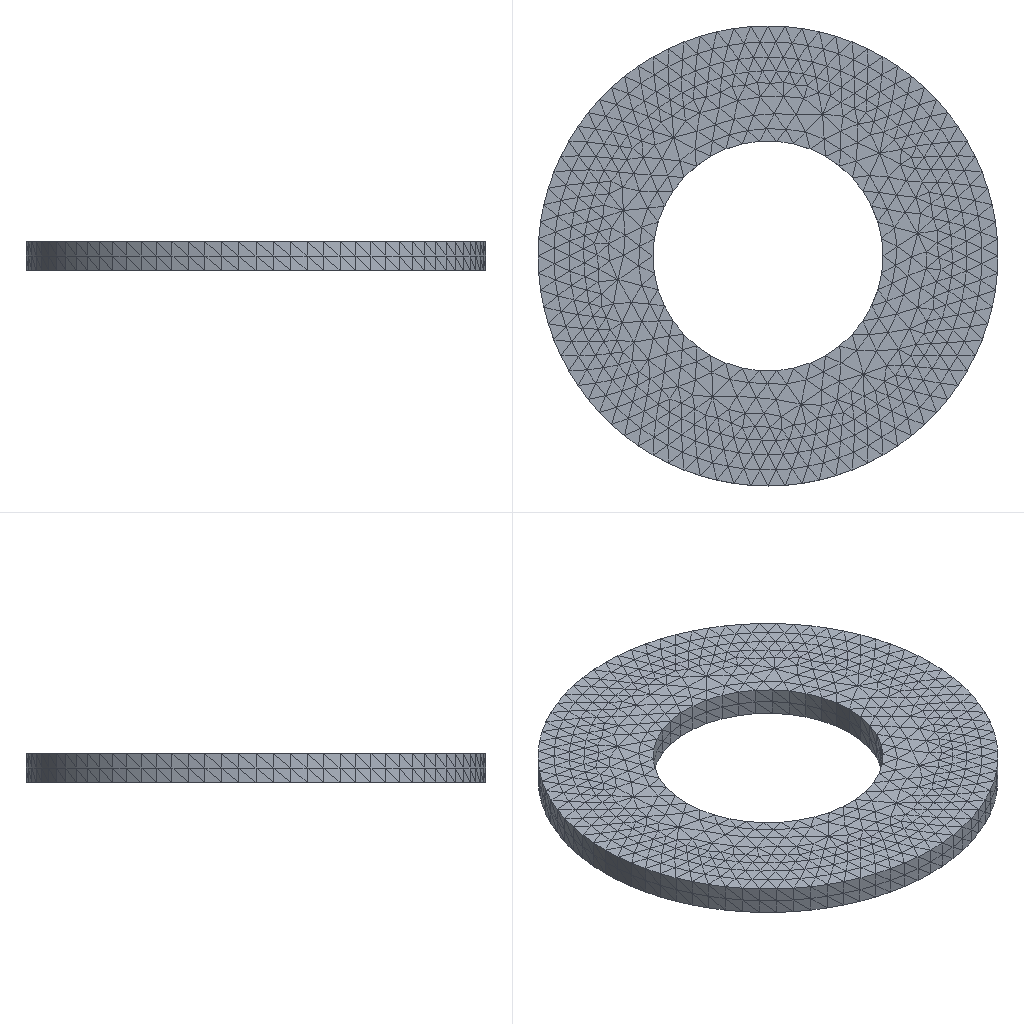Simulation study | abaqus
Notes in the study folder:
14 annular disk
job_status=None
Umax_mm=0.00147959
S_Mises_max_MPa=7.88113
Set-up summary:
category,name,step,type,value,unit,region
solver,abaqus,,Abaqus/CAE 2024
units,mm-N-s-tonne (MPa),,inferred,E=210000 density=7.85e-09
analysis,Step-1,,static,time_period=1
mesh,nodes,,,12333
mesh,elements,,,7205
element_type,C3D10,,,7205
material,Steel,,E,210000
material,Steel,,nu,0.3
material,Steel,,density,7.85e-09
section,Steel,,solid section,,,_PickedSet2
load,P,Step-1,pressure,0.15,,PRESS
bc,BC,Step-1,encastre,[dofs=ENCASTRE],,FIXED
Abaqus input file, long lists of numbers shortened:
*Heading
** Job name: deck Model name: M14
** Generated by: Abaqus/CAE 2024
*Preprint, echo=NO, model=NO, history=NO, contact=NO
**
** PARTS
**
*Part, name=P
*Node
      1,          20.,           0.,           5.
      2,          20.,           0.,           0.
** (12331 more lines like these left out)
*Element, type=C3D10
   1,  1303,  1304,   452,  1305,  1916,  1915,  1914,  1918,  1917,  1919
   2,  1303,  1306,  1120,  1307,  1922,  1921,  1920,  1924,  1923,  1925
** (7203 more lines like these left out)
*Nset, nset=_PickedSet2, internal, generate
     1,  12333,      1
*Elset, elset=_PickedSet2, internal, generate
    1,  7205,     1
** Section: Sec
*Solid Section, elset=_PickedSet2, material=Steel
,
*End Part
**
**
** ASSEMBLY
**
*Assembly, name=Assembly
**
*Instance, name=I, part=P
*End Instance
**
*Nset, nset=FIXED, instance=I
     1,     2,     5,     6,     7,     8,     9,    10,    11,    12,    13,    14,    15,    16,    17,    18
    19,    20,    21,    22,    23,    24,    25,    26,    27,    28,    29,    30,    31,    32,    33,    34
** (25 more lines like these left out)
*Elset, elset=FIXED, instance=I
  110,  782,  798,  959, 1212, 1397, 1451, 1493, 1630, 1659, 1667, 1701, 1765, 1766, 1822, 1845
 1851, 1861, 1863, 1915, 1917, 1931, 1932, 1946, 1948, 1949, 1952, 1955, 1956, 1964, 1974, 1990
** (9 more lines like these left out)
*Elset, elset=_PRESS_S2, internal, instance=I
   77,  110,  815, 1659, 1665, 1949, 1990, 2108, 2173, 2322, 2345, 2364, 2510, 2529, 2591, 2618
 2680, 2682, 2685, 2764, 2914, 2992, 3210, 3277, 3629, 3735, 3740, 3819, 4110, 4581, 4920, 4948
** (1 more lines like these left out)
*Elset, elset=_PRESS_S3, internal, instance=I
  132,  133,  151,  217,  228,  345,  422,  473,  565,  599,  610,  692,  721,  802,  922,  965
  968, 1069, 1155, 1157, 1162, 1171, 1175, 1250, 1276, 1277, 1353, 1380, 1405, 1408, 1514, 1570
** (56 more lines like these left out)
*Elset, elset=_PRESS_S4, internal, instance=I
  669,  795, 1041, 1275, 1315, 1332, 1812, 2058, 2073, 2098, 2107, 2115, 2253, 2538, 2830, 2854
 3101, 3116, 3472, 3551, 3557, 3778, 4094, 4275, 4349, 4443, 4502, 4741, 5007, 5276, 5420, 5456
** (1 more lines like these left out)
*Elset, elset=_PRESS_S1, internal, instance=I
 1050, 1073, 1116, 1192, 1221, 1537, 1580, 1630, 1845, 1851, 1908, 1915, 2006, 2077, 2078, 2102
 2175, 2178, 2189, 2191, 2200, 2234, 2393, 2403, 2625, 2725, 3004, 3011, 3087, 3148, 3358, 3373
** (2 more lines like these left out)
*Surface, type=ELEMENT, name=PRESS
_PRESS_S2, S2
_PRESS_S3, S3
_PRESS_S4, S4
_PRESS_S1, S1
*End Assembly
**
** MATERIALS
**
*Material, name=Steel
*Density
 7.85e-09,
*Elastic
210000., 0.3
** ----------------------------------------------------------------
**
** STEP: Step-1
**
*Step, name=Step-1, nlgeom=NO
*Static
1., 1., 1e-05, 1.
**
** BOUNDARY CONDITIONS
**
** Name: BC Type: Symmetry/Antisymmetry/Encastre
*Boundary
FIXED, ENCASTRE
**
** LOADS
**
** Name: P   Type: Pressure
*Dsload
PRESS, P, 0.15
**
** OUTPUT REQUESTS
**
*Restart, write, frequency=0
**
** FIELD OUTPUT: F-Output-1
**
*Output, field, variable=PRESELECT
**
** HISTORY OUTPUT: H-Output-1
**
*Output, history, variable=PRESELECT
*End Step
Results summary:
result,odb.job_status,,,JOB_STATUS_COMPLETED_SUCCESSFULLY,"consistent, unstated (Abaqus has no unit system)"
result,steps[0].procedure,Step-1,,*STATIC,"consistent, unstated (Abaqus has no unit system)"
result,steps[0].time_period,Step-1,,1,"consistent, unstated (Abaqus has no unit system)"
result,steps[0].n_frames,Step-1,,2,"consistent, unstated (Abaqus has no unit system)"
result,steps[0].last_frame.id,Step-1,,1,"consistent, unstated (Abaqus has no unit system)"
result,steps[0].last_frame.value,Step-1,,1,"consistent, unstated (Abaqus has no unit system)"
result,steps[0].last_frame.description,Step-1,,Increment      1: Step Time =    1.000,"consistent, unstated (Abaqus has no unit system)"
result,steps[0].completed,Step-1,,True,"consistent, unstated (Abaqus has no unit system)"
result,steps[0].max_U_magnitude,Step-1,,0.00148,"consistent, unstated (Abaqus has no unit system)"
result,steps[0].max_S_mises,Step-1,,7.881,"consistent, unstated (Abaqus has no unit system)"
result,steps[0].RF_sum[1],Step-1,,1.28746e-05,"consistent, unstated (Abaqus has no unit system)"
result,steps[0].RF_sum[2],Step-1,,-2.38419e-05,"consistent, unstated (Abaqus has no unit system)"
result,steps[0].RF_sum[3],Step-1,,565.487,"consistent, unstated (Abaqus has no unit system)"
result,steps[1].procedure,Step-1,,*STATIC,"consistent, unstated (Abaqus has no unit system)"
result,steps[1].time_period,Step-1,,1,"consistent, unstated (Abaqus has no unit system)"
result,steps[1].n_frames,Step-1,,2,"consistent, unstated (Abaqus has no unit system)"
result,steps[1].last_frame.id,Step-1,,1,"consistent, unstated (Abaqus has no unit system)"
result,steps[1].last_frame.value,Step-1,,1,"consistent, unstated (Abaqus has no unit system)"
result,steps[1].last_frame.description,Step-1,,Increment      1: Step Time =    1.000,"consistent, unstated (Abaqus has no unit system)"
result,steps[1].completed,Step-1,,True,"consistent, unstated (Abaqus has no unit system)"
result,steps[1].max_U_magnitude,Step-1,,0.00148,"consistent, unstated (Abaqus has no unit system)"
result,steps[1].max_S_mises,Step-1,,7.881,"consistent, unstated (Abaqus has no unit system)"
result,steps[1].RF_sum[1],Step-1,,1.28746e-05,"consistent, unstated (Abaqus has no unit system)"
result,steps[1].RF_sum[2],Step-1,,-2.38419e-05,"consistent, unstated (Abaqus has no unit system)"
result,steps[1].RF_sum[3],Step-1,,565.487,"consistent, unstated (Abaqus has no unit system)"